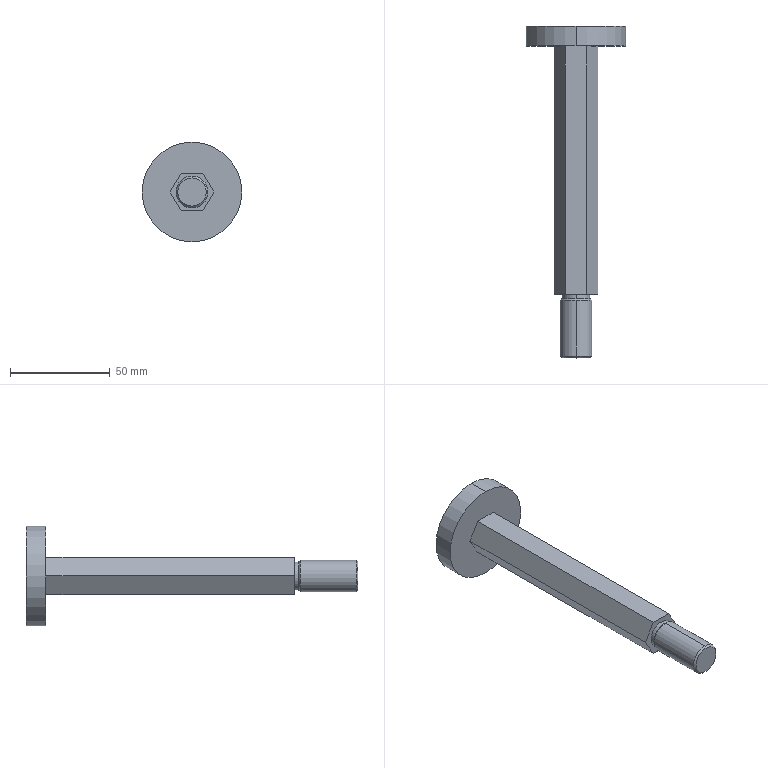Part | SolidWorks | features BaseBody 1 | 1 solid | 21 faces | box 50 x 166.5 x 50 mm | volume 64845 mm3 | plane 11 | cylinder 6 | cone 4 | commonest cylinder face diameters 14 x2 16 x2 50 x2
STEP:
#1=CARTESIAN_POINT('',(225.,248.5,159.621));
#2=VERTEX_POINT('',#1);
#3=CARTESIAN_POINT('',(225.,248.5,109.621));
#4=VERTEX_POINT('',#3);
#5=CARTESIAN_POINT('',(225.,248.5,134.621));
#6=DIRECTION('',(0.,1.,0.));
#7=DIRECTION('',(0.,0.,1.));
#8=AXIS2_PLACEMENT_3D('',#5,#6,#7);
#9=CIRCLE('',#8,25.);
#10=EDGE_CURVE('',#2,#4,#9,.T.);
#11=ORIENTED_EDGE('',*,*,#10,.T.);
#12=CARTESIAN_POINT('',(225.,258.5,109.621));
#13=VERTEX_POINT('',#12);
#14=CARTESIAN_POINT('',(225.,253.5,109.621));
#15=DIRECTION('',(0.,1.,0.));
#16=VECTOR('',#15,1000.);
#17=LINE('',#14,#16);
#18=EDGE_CURVE('',#4,#13,#17,.T.);
#19=ORIENTED_EDGE('',*,*,#18,.T.);
#20=CARTESIAN_POINT('',(225.,258.5,159.621));
#21=VERTEX_POINT('',#20);
#22=CARTESIAN_POINT('',(225.,258.5,134.621));
#23=DIRECTION('',(0.,1.,0.));
#24=DIRECTION('',(0.,0.,1.));
#25=AXIS2_PLACEMENT_3D('',#22,#23,#24);
#26=CIRCLE('',#25,25.);
#27=EDGE_CURVE('',#21,#13,#26,.T.);
#28=ORIENTED_EDGE('',*,*,#27,.F.);
#29=CARTESIAN_POINT('',(225.,253.5,159.621));
#30=DIRECTION('',(0.,1.,0.));
#31=VECTOR('',#30,1000.);
#32=LINE('',#29,#31);
#33=EDGE_CURVE('',#2,#21,#32,.T.);
#34=ORIENTED_EDGE('',*,*,#33,.F.);
#35=EDGE_LOOP('',(#11,#19,#28,#34));
#36=FACE_OUTER_BOUND('',#35,.T.);
#37=CARTESIAN_POINT('',(225.,253.5,134.621));
#38=DIRECTION('',(0.,1.,0.));
#39=DIRECTION('',(0.,0.,1.));
#40=AXIS2_PLACEMENT_3D('',#37,#38,#39);
#41=CYLINDRICAL_SURFACE('',#40,25.);
#42=ADVANCED_FACE('',(#36),#41,.T.);
#43=CARTESIAN_POINT('',(225.,121.75,141.621));
#44=VERTEX_POINT('',#43);
#45=CARTESIAN_POINT('',(225.,121.75,127.621));
#46=VERTEX_POINT('',#45);
#47=CARTESIAN_POINT('',(225.,121.75,134.621));
#48=DIRECTION('',(0.,1.,0.));
#49=DIRECTION('',(0.,0.,1.));
#50=AXIS2_PLACEMENT_3D('',#47,#48,#49);
#51=CIRCLE('',#50,7.);
#52=EDGE_CURVE('',#44,#46,#51,.T.);
#53=ORIENTED_EDGE('',*,*,#52,.T.);
#54=CARTESIAN_POINT('',(225.,124.,127.621));
#55=VERTEX_POINT('',#54);
#56=CARTESIAN_POINT('',(225.,122.875,127.621));
#57=DIRECTION('',(0.,1.,0.));
#58=VECTOR('',#57,1000.);
#59=LINE('',#56,#58);
#60=EDGE_CURVE('',#46,#55,#59,.T.);
#61=ORIENTED_EDGE('',*,*,#60,.T.);
#62=CARTESIAN_POINT('',(225.,124.,141.621));
#63=VERTEX_POINT('',#62);
#64=CARTESIAN_POINT('',(225.,124.,134.621));
#65=DIRECTION('',(0.,1.,0.));
#66=DIRECTION('',(0.,0.,1.));
#67=AXIS2_PLACEMENT_3D('',#64,#65,#66);
#68=CIRCLE('',#67,7.);
#69=EDGE_CURVE('',#63,#55,#68,.T.);
#70=ORIENTED_EDGE('',*,*,#69,.F.);
#71=CARTESIAN_POINT('',(225.,122.875,141.621));
#72=DIRECTION('',(0.,1.,0.));
#73=VECTOR('',#72,1000.);
#74=LINE('',#71,#73);
#75=EDGE_CURVE('',#44,#63,#74,.T.);
#76=ORIENTED_EDGE('',*,*,#75,.F.);
#77=EDGE_LOOP('',(#53,#61,#70,#76));
#78=FACE_OUTER_BOUND('',#77,.T.);
#79=CARTESIAN_POINT('',(225.,122.875,134.621));
#80=DIRECTION('',(0.,1.,0.));
#81=DIRECTION('',(0.,0.,1.));
#82=AXIS2_PLACEMENT_3D('',#79,#80,#81);
#83=CYLINDRICAL_SURFACE('',#82,7.);
#84=ADVANCED_FACE('',(#78),#83,.T.);
#85=CARTESIAN_POINT('',(225.,121.75,141.701));
#86=VERTEX_POINT('',#85);
#87=CARTESIAN_POINT('',(225.,121.75,127.541));
#88=VERTEX_POINT('',#87);
#89=CARTESIAN_POINT('',(225.,121.75,134.621));
#90=DIRECTION('',(0.,1.,0.));
#91=DIRECTION('',(0.,0.,-1.));
#92=AXIS2_PLACEMENT_3D('',#89,#90,#91);
#93=CIRCLE('',#92,7.08);
#94=EDGE_CURVE('',#86,#88,#93,.T.);
#95=ORIENTED_EDGE('',*,*,#94,.F.);
#96=CARTESIAN_POINT('',(225.,120.83,142.621));
#97=VERTEX_POINT('',#96);
#98=CARTESIAN_POINT('',(225.,120.83,142.621));
#99=DIRECTION('',(0.,-0.7071,0.7071));
#100=VECTOR('',#99,1000.);
#101=LINE('',#98,#100);
#102=EDGE_CURVE('',#86,#97,#101,.T.);
#103=ORIENTED_EDGE('',*,*,#102,.T.);
#104=CARTESIAN_POINT('',(225.,120.83,126.621));
#105=VERTEX_POINT('',#104);
#106=CARTESIAN_POINT('',(225.,120.83,134.621));
#107=DIRECTION('',(0.,1.,0.));
#108=DIRECTION('',(-0.5,0.,0.866));
#109=AXIS2_PLACEMENT_3D('',#106,#107,#108);
#110=CIRCLE('',#109,8.);
#111=EDGE_CURVE('',#97,#105,#110,.T.);
#112=ORIENTED_EDGE('',*,*,#111,.T.);
#113=CARTESIAN_POINT('',(225.,120.83,126.621));
#114=DIRECTION('',(0.,-0.7071,-0.7071));
#115=VECTOR('',#114,1000.);
#116=LINE('',#113,#115);
#117=EDGE_CURVE('',#88,#105,#116,.T.);
#118=ORIENTED_EDGE('',*,*,#117,.F.);
#119=EDGE_LOOP('',(#95,#103,#112,#118));
#120=FACE_OUTER_BOUND('',#119,.T.);
#121=CARTESIAN_POINT('',(225.,120.83,134.621));
#122=DIRECTION('',(0.,-1.,0.));
#123=DIRECTION('',(0.,0.,-1.));
#124=AXIS2_PLACEMENT_3D('',#121,#122,#123);
#125=CONICAL_SURFACE('',#124,8.,0.7854);
#126=ADVANCED_FACE('',(#120),#125,.T.);
#127=CARTESIAN_POINT('',(225.,92.92,142.621));
#128=VERTEX_POINT('',#127);
#129=CARTESIAN_POINT('',(225.,92.92,126.621));
#130=VERTEX_POINT('',#129);
#131=CARTESIAN_POINT('',(225.,92.92,134.621));
#132=DIRECTION('',(0.,1.,0.));
#133=DIRECTION('',(0.,0.,1.));
#134=AXIS2_PLACEMENT_3D('',#131,#132,#133);
#135=CIRCLE('',#134,8.);
#136=EDGE_CURVE('',#128,#130,#135,.T.);
#137=ORIENTED_EDGE('',*,*,#136,.T.);
#138=CARTESIAN_POINT('',(225.,106.875,126.621));
#139=DIRECTION('',(0.,1.,0.));
#140=VECTOR('',#139,1000.);
#141=LINE('',#138,#140);
#142=EDGE_CURVE('',#130,#105,#141,.T.);
#143=ORIENTED_EDGE('',*,*,#142,.T.);
#144=ORIENTED_EDGE('',*,*,#111,.F.);
#145=CARTESIAN_POINT('',(225.,106.875,142.621));
#146=DIRECTION('',(0.,1.,0.));
#147=VECTOR('',#146,1000.);
#148=LINE('',#145,#147);
#149=EDGE_CURVE('',#128,#97,#148,.T.);
#150=ORIENTED_EDGE('',*,*,#149,.F.);
#151=EDGE_LOOP('',(#137,#143,#144,#150));
#152=FACE_OUTER_BOUND('',#151,.T.);
#153=CARTESIAN_POINT('',(225.,106.875,134.621));
#154=DIRECTION('',(0.,1.,0.));
#155=DIRECTION('',(0.,0.,1.));
#156=AXIS2_PLACEMENT_3D('',#153,#154,#155);
#157=CYLINDRICAL_SURFACE('',#156,8.);
#158=ADVANCED_FACE('',(#152),#157,.T.);
#159=CARTESIAN_POINT('',(225.,92.,141.701));
#160=VERTEX_POINT('',#159);
#161=CARTESIAN_POINT('',(225.,92.,127.541));
#162=VERTEX_POINT('',#161);
#163=CARTESIAN_POINT('',(225.,92.,134.621));
#164=DIRECTION('',(0.,1.,0.));
#165=DIRECTION('',(0.,0.,1.));
#166=AXIS2_PLACEMENT_3D('',#163,#164,#165);
#167=CIRCLE('',#166,7.08);
#168=EDGE_CURVE('',#160,#162,#167,.T.);
#169=ORIENTED_EDGE('',*,*,#168,.T.);
#170=CARTESIAN_POINT('',(225.,92.92,126.621));
#171=DIRECTION('',(0.,0.7071,-0.7071));
#172=VECTOR('',#171,1000.);
#173=LINE('',#170,#172);
#174=EDGE_CURVE('',#162,#130,#173,.T.);
#175=ORIENTED_EDGE('',*,*,#174,.T.);
#176=ORIENTED_EDGE('',*,*,#136,.F.);
#177=CARTESIAN_POINT('',(225.,92.92,142.621));
#178=DIRECTION('',(0.,0.7071,0.7071));
#179=VECTOR('',#178,1000.);
#180=LINE('',#177,#179);
#181=EDGE_CURVE('',#160,#128,#180,.T.);
#182=ORIENTED_EDGE('',*,*,#181,.F.);
#183=EDGE_LOOP('',(#169,#175,#176,#182));
#184=FACE_OUTER_BOUND('',#183,.T.);
#185=CARTESIAN_POINT('',(225.,92.92,134.621));
#186=DIRECTION('',(0.,1.,0.));
#187=DIRECTION('',(0.,0.,1.));
#188=AXIS2_PLACEMENT_3D('',#185,#186,#187);
#189=CONICAL_SURFACE('',#188,8.,0.7854);
#190=ADVANCED_FACE('',(#184),#189,.T.);
#191=ORIENTED_EDGE('',*,*,#27,.T.);
#192=CARTESIAN_POINT('',(225.,258.5,134.621));
#193=DIRECTION('',(0.,1.,0.));
#194=DIRECTION('',(0.,0.,1.));
#195=AXIS2_PLACEMENT_3D('',#192,#193,#194);
#196=CIRCLE('',#195,25.);
#197=EDGE_CURVE('',#13,#21,#196,.T.);
#198=ORIENTED_EDGE('',*,*,#197,.T.);
#199=EDGE_LOOP('',(#191,#198));
#200=FACE_OUTER_BOUND('',#199,.T.);
#201=CARTESIAN_POINT('',(235.825,258.5,140.871));
#202=DIRECTION('',(0.,1.,0.));
#203=DIRECTION('',(0.,0.,1.));
#204=AXIS2_PLACEMENT_3D('',#201,#202,#203);
#205=PLANE('',#204);
#206=ADVANCED_FACE('',(#200),#205,.T.);
#207=ORIENTED_EDGE('',*,*,#18,.F.);
#208=CARTESIAN_POINT('',(225.,248.5,134.621));
#209=DIRECTION('',(0.,1.,0.));
#210=DIRECTION('',(0.,0.,1.));
#211=AXIS2_PLACEMENT_3D('',#208,#209,#210);
#212=CIRCLE('',#211,25.);
#213=EDGE_CURVE('',#4,#2,#212,.T.);
#214=ORIENTED_EDGE('',*,*,#213,.T.);
#215=ORIENTED_EDGE('',*,*,#33,.T.);
#216=ORIENTED_EDGE('',*,*,#197,.F.);
#217=EDGE_LOOP('',(#207,#214,#215,#216));
#218=FACE_OUTER_BOUND('',#217,.T.);
#219=CARTESIAN_POINT('',(225.,253.5,134.621));
#220=DIRECTION('',(0.,1.,0.));
#221=DIRECTION('',(0.,0.,1.));
#222=AXIS2_PLACEMENT_3D('',#219,#220,#221);
#223=CYLINDRICAL_SURFACE('',#222,25.);
#224=ADVANCED_FACE('',(#218),#223,.T.);
#225=CARTESIAN_POINT('',(214.03,248.5,134.621));
#226=VERTEX_POINT('',#225);
#227=CARTESIAN_POINT('',(219.515,248.5,144.121));
#228=VERTEX_POINT('',#227);
#229=CARTESIAN_POINT('',(214.03,248.5,134.621));
#230=DIRECTION('',(0.5,0.,0.866));
#231=VECTOR('',#230,1000.);
#232=LINE('',#229,#231);
#233=EDGE_CURVE('',#226,#228,#232,.T.);
#234=ORIENTED_EDGE('',*,*,#233,.T.);
#235=CARTESIAN_POINT('',(230.485,248.5,144.121));
#236=VERTEX_POINT('',#235);
#237=CARTESIAN_POINT('',(242.407,248.5,144.121));
#238=DIRECTION('',(1.,0.,0.));
#239=VECTOR('',#238,1000.);
#240=LINE('',#237,#239);
#241=EDGE_CURVE('',#228,#236,#240,.T.);
#242=ORIENTED_EDGE('',*,*,#241,.T.);
#243=CARTESIAN_POINT('',(235.97,248.5,134.621));
#244=VERTEX_POINT('',#243);
#245=CARTESIAN_POINT('',(230.485,248.5,144.121));
#246=DIRECTION('',(0.5,0.,-0.866));
#247=VECTOR('',#246,1000.);
#248=LINE('',#245,#247);
#249=EDGE_CURVE('',#236,#244,#248,.T.);
#250=ORIENTED_EDGE('',*,*,#249,.T.);
#251=CARTESIAN_POINT('',(230.485,248.5,125.121));
#252=VERTEX_POINT('',#251);
#253=CARTESIAN_POINT('',(235.97,248.5,134.621));
#254=DIRECTION('',(-0.5,0.,-0.866));
#255=VECTOR('',#254,1000.);
#256=LINE('',#253,#255);
#257=EDGE_CURVE('',#244,#252,#256,.T.);
#258=ORIENTED_EDGE('',*,*,#257,.T.);
#259=CARTESIAN_POINT('',(219.515,248.5,125.121));
#260=VERTEX_POINT('',#259);
#261=CARTESIAN_POINT('',(242.407,248.5,125.121));
#262=DIRECTION('',(-1.,0.,0.));
#263=VECTOR('',#262,1000.);
#264=LINE('',#261,#263);
#265=EDGE_CURVE('',#252,#260,#264,.T.);
#266=ORIENTED_EDGE('',*,*,#265,.T.);
#267=CARTESIAN_POINT('',(219.515,248.5,125.121));
#268=DIRECTION('',(-0.5,0.,0.866));
#269=VECTOR('',#268,1000.);
#270=LINE('',#267,#269);
#271=EDGE_CURVE('',#260,#226,#270,.T.);
#272=ORIENTED_EDGE('',*,*,#271,.T.);
#273=EDGE_LOOP('',(#234,#242,#250,#258,#266,#272));
#274=FACE_BOUND('',#273,.T.);
#275=ORIENTED_EDGE('',*,*,#10,.F.);
#276=ORIENTED_EDGE('',*,*,#213,.F.);
#277=EDGE_LOOP('',(#275,#276));
#278=FACE_OUTER_BOUND('',#277,.T.);
#279=CARTESIAN_POINT('',(242.407,248.5,144.671));
#280=DIRECTION('',(0.,-1.,0.));
#281=DIRECTION('',(0.,0.,-1.));
#282=AXIS2_PLACEMENT_3D('',#279,#280,#281);
#283=PLANE('',#282);
#284=ADVANCED_FACE('',(#274,#278),#283,.T.);
#285=CARTESIAN_POINT('',(230.485,124.,144.121));
#286=VERTEX_POINT('',#285);
#287=CARTESIAN_POINT('',(219.515,124.,144.121));
#288=VERTEX_POINT('',#287);
#289=CARTESIAN_POINT('',(219.515,124.,144.121));
#290=DIRECTION('',(-1.,0.,0.));
#291=VECTOR('',#290,1000.);
#292=LINE('',#289,#291);
#293=EDGE_CURVE('',#286,#288,#292,.T.);
#294=ORIENTED_EDGE('',*,*,#293,.F.);
#295=CARTESIAN_POINT('',(230.485,124.,144.121));
#296=DIRECTION('',(0.,-1.,0.));
#297=VECTOR('',#296,1000.);
#298=LINE('',#295,#297);
#299=EDGE_CURVE('',#236,#286,#298,.T.);
#300=ORIENTED_EDGE('',*,*,#299,.F.);
#301=ORIENTED_EDGE('',*,*,#241,.F.);
#302=CARTESIAN_POINT('',(219.515,124.,144.121));
#303=DIRECTION('',(0.,1.,0.));
#304=VECTOR('',#303,1000.);
#305=LINE('',#302,#304);
#306=EDGE_CURVE('',#288,#228,#305,.T.);
#307=ORIENTED_EDGE('',*,*,#306,.F.);
#308=EDGE_LOOP('',(#294,#300,#301,#307));
#309=FACE_OUTER_BOUND('',#308,.T.);
#310=CARTESIAN_POINT('',(219.515,124.,144.121));
#311=DIRECTION('',(0.,0.,-1.));
#312=DIRECTION('',(-1.,0.,0.));
#313=AXIS2_PLACEMENT_3D('',#310,#311,#312);
#314=PLANE('',#313);
#315=ADVANCED_FACE('',(#309),#314,.F.);
#316=CARTESIAN_POINT('',(214.03,124.,134.621));
#317=VERTEX_POINT('',#316);
#318=CARTESIAN_POINT('',(214.03,124.,134.621));
#319=DIRECTION('',(-0.5,0.,-0.866));
#320=VECTOR('',#319,1000.);
#321=LINE('',#318,#320);
#322=EDGE_CURVE('',#288,#317,#321,.T.);
#323=ORIENTED_EDGE('',*,*,#322,.F.);
#324=ORIENTED_EDGE('',*,*,#306,.T.);
#325=ORIENTED_EDGE('',*,*,#233,.F.);
#326=CARTESIAN_POINT('',(214.03,124.,134.621));
#327=DIRECTION('',(0.,1.,0.));
#328=VECTOR('',#327,1000.);
#329=LINE('',#326,#328);
#330=EDGE_CURVE('',#317,#226,#329,.T.);
#331=ORIENTED_EDGE('',*,*,#330,.F.);
#332=EDGE_LOOP('',(#323,#324,#325,#331));
#333=FACE_OUTER_BOUND('',#332,.T.);
#334=CARTESIAN_POINT('',(214.03,124.,134.621));
#335=DIRECTION('',(0.866,0.,-0.5));
#336=DIRECTION('',(-0.5,0.,-0.866));
#337=AXIS2_PLACEMENT_3D('',#334,#335,#336);
#338=PLANE('',#337);
#339=ADVANCED_FACE('',(#333),#338,.F.);
#340=CARTESIAN_POINT('',(219.515,124.,125.121));
#341=VERTEX_POINT('',#340);
#342=CARTESIAN_POINT('',(219.515,124.,125.121));
#343=DIRECTION('',(0.5,0.,-0.866));
#344=VECTOR('',#343,1000.);
#345=LINE('',#342,#344);
#346=EDGE_CURVE('',#317,#341,#345,.T.);
#347=ORIENTED_EDGE('',*,*,#346,.F.);
#348=ORIENTED_EDGE('',*,*,#330,.T.);
#349=ORIENTED_EDGE('',*,*,#271,.F.);
#350=CARTESIAN_POINT('',(219.515,124.,125.121));
#351=DIRECTION('',(0.,1.,0.));
#352=VECTOR('',#351,1000.);
#353=LINE('',#350,#352);
#354=EDGE_CURVE('',#341,#260,#353,.T.);
#355=ORIENTED_EDGE('',*,*,#354,.F.);
#356=EDGE_LOOP('',(#347,#348,#349,#355));
#357=FACE_OUTER_BOUND('',#356,.T.);
#358=CARTESIAN_POINT('',(219.515,124.,125.121));
#359=DIRECTION('',(0.866,0.,0.5));
#360=DIRECTION('',(0.5,0.,-0.866));
#361=AXIS2_PLACEMENT_3D('',#358,#359,#360);
#362=PLANE('',#361);
#363=ADVANCED_FACE('',(#357),#362,.F.);
#364=CARTESIAN_POINT('',(230.485,124.,125.121));
#365=VERTEX_POINT('',#364);
#366=CARTESIAN_POINT('',(230.485,124.,125.121));
#367=DIRECTION('',(1.,0.,0.));
#368=VECTOR('',#367,1000.);
#369=LINE('',#366,#368);
#370=EDGE_CURVE('',#341,#365,#369,.T.);
#371=ORIENTED_EDGE('',*,*,#370,.F.);
#372=ORIENTED_EDGE('',*,*,#354,.T.);
#373=ORIENTED_EDGE('',*,*,#265,.F.);
#374=CARTESIAN_POINT('',(230.485,124.,125.121));
#375=DIRECTION('',(0.,1.,0.));
#376=VECTOR('',#375,1000.);
#377=LINE('',#374,#376);
#378=EDGE_CURVE('',#365,#252,#377,.T.);
#379=ORIENTED_EDGE('',*,*,#378,.F.);
#380=EDGE_LOOP('',(#371,#372,#373,#379));
#381=FACE_OUTER_BOUND('',#380,.T.);
#382=CARTESIAN_POINT('',(230.485,124.,125.121));
#383=DIRECTION('',(0.,0.,1.));
#384=DIRECTION('',(1.,0.,0.));
#385=AXIS2_PLACEMENT_3D('',#382,#383,#384);
#386=PLANE('',#385);
#387=ADVANCED_FACE('',(#381),#386,.F.);
#388=CARTESIAN_POINT('',(235.97,124.,134.621));
#389=VERTEX_POINT('',#388);
#390=CARTESIAN_POINT('',(235.97,124.,134.621));
#391=DIRECTION('',(0.5,0.,0.866));
#392=VECTOR('',#391,1000.);
#393=LINE('',#390,#392);
#394=EDGE_CURVE('',#365,#389,#393,.T.);
#395=ORIENTED_EDGE('',*,*,#394,.F.);
#396=ORIENTED_EDGE('',*,*,#378,.T.);
#397=ORIENTED_EDGE('',*,*,#257,.F.);
#398=CARTESIAN_POINT('',(235.97,124.,134.621));
#399=DIRECTION('',(0.,1.,0.));
#400=VECTOR('',#399,1000.);
#401=LINE('',#398,#400);
#402=EDGE_CURVE('',#389,#244,#401,.T.);
#403=ORIENTED_EDGE('',*,*,#402,.F.);
#404=EDGE_LOOP('',(#395,#396,#397,#403));
#405=FACE_OUTER_BOUND('',#404,.T.);
#406=CARTESIAN_POINT('',(235.97,124.,134.621));
#407=DIRECTION('',(-0.866,0.,0.5));
#408=DIRECTION('',(0.5,0.,0.866));
#409=AXIS2_PLACEMENT_3D('',#406,#407,#408);
#410=PLANE('',#409);
#411=ADVANCED_FACE('',(#405),#410,.F.);
#412=CARTESIAN_POINT('',(230.485,124.,144.121));
#413=DIRECTION('',(-0.5,0.,0.866));
#414=VECTOR('',#413,1000.);
#415=LINE('',#412,#414);
#416=EDGE_CURVE('',#389,#286,#415,.T.);
#417=ORIENTED_EDGE('',*,*,#416,.F.);
#418=ORIENTED_EDGE('',*,*,#402,.T.);
#419=ORIENTED_EDGE('',*,*,#249,.F.);
#420=ORIENTED_EDGE('',*,*,#299,.T.);
#421=EDGE_LOOP('',(#417,#418,#419,#420));
#422=FACE_OUTER_BOUND('',#421,.T.);
#423=CARTESIAN_POINT('',(230.485,124.,144.121));
#424=DIRECTION('',(-0.866,0.,-0.5));
#425=DIRECTION('',(-0.5,0.,0.866));
#426=AXIS2_PLACEMENT_3D('',#423,#424,#425);
#427=PLANE('',#426);
#428=ADVANCED_FACE('',(#422),#427,.F.);
#429=ORIENTED_EDGE('',*,*,#416,.T.);
#430=ORIENTED_EDGE('',*,*,#293,.T.);
#431=ORIENTED_EDGE('',*,*,#322,.T.);
#432=ORIENTED_EDGE('',*,*,#346,.T.);
#433=ORIENTED_EDGE('',*,*,#370,.T.);
#434=ORIENTED_EDGE('',*,*,#394,.T.);
#435=EDGE_LOOP('',(#429,#430,#431,#432,#433,#434));
#436=FACE_OUTER_BOUND('',#435,.T.);
#437=ORIENTED_EDGE('',*,*,#69,.T.);
#438=CARTESIAN_POINT('',(225.,124.,134.621));
#439=DIRECTION('',(0.,1.,0.));
#440=DIRECTION('',(0.,0.,1.));
#441=AXIS2_PLACEMENT_3D('',#438,#439,#440);
#442=CIRCLE('',#441,7.);
#443=EDGE_CURVE('',#55,#63,#442,.T.);
#444=ORIENTED_EDGE('',*,*,#443,.T.);
#445=EDGE_LOOP('',(#437,#444));
#446=FACE_BOUND('',#445,.T.);
#447=CARTESIAN_POINT('',(234.613,124.,140.171));
#448=DIRECTION('',(0.,-1.,0.));
#449=DIRECTION('',(0.,0.,-1.));
#450=AXIS2_PLACEMENT_3D('',#447,#448,#449);
#451=PLANE('',#450);
#452=ADVANCED_FACE('',(#436,#446),#451,.T.);
#453=ORIENTED_EDGE('',*,*,#60,.F.);
#454=CARTESIAN_POINT('',(225.,121.75,134.621));
#455=DIRECTION('',(0.,1.,0.));
#456=DIRECTION('',(0.,0.,1.));
#457=AXIS2_PLACEMENT_3D('',#454,#455,#456);
#458=CIRCLE('',#457,7.);
#459=EDGE_CURVE('',#46,#44,#458,.T.);
#460=ORIENTED_EDGE('',*,*,#459,.T.);
#461=ORIENTED_EDGE('',*,*,#75,.T.);
#462=ORIENTED_EDGE('',*,*,#443,.F.);
#463=EDGE_LOOP('',(#453,#460,#461,#462));
#464=FACE_OUTER_BOUND('',#463,.T.);
#465=CARTESIAN_POINT('',(225.,122.875,134.621));
#466=DIRECTION('',(0.,1.,0.));
#467=DIRECTION('',(0.,0.,1.));
#468=AXIS2_PLACEMENT_3D('',#465,#466,#467);
#469=CYLINDRICAL_SURFACE('',#468,7.);
#470=ADVANCED_FACE('',(#464),#469,.T.);
#471=CARTESIAN_POINT('',(225.,121.75,134.621));
#472=DIRECTION('',(0.,1.,0.));
#473=DIRECTION('',(0.,0.,-1.));
#474=AXIS2_PLACEMENT_3D('',#471,#472,#473);
#475=CIRCLE('',#474,7.08);
#476=EDGE_CURVE('',#88,#86,#475,.T.);
#477=ORIENTED_EDGE('',*,*,#476,.T.);
#478=ORIENTED_EDGE('',*,*,#94,.T.);
#479=EDGE_LOOP('',(#477,#478));
#480=FACE_OUTER_BOUND('',#479,.T.);
#481=ORIENTED_EDGE('',*,*,#52,.F.);
#482=ORIENTED_EDGE('',*,*,#459,.F.);
#483=EDGE_LOOP('',(#481,#482));
#484=FACE_BOUND('',#483,.T.);
#485=CARTESIAN_POINT('',(231.097,121.75,138.141));
#486=DIRECTION('',(0.,1.,0.));
#487=DIRECTION('',(0.,0.,1.));
#488=AXIS2_PLACEMENT_3D('',#485,#486,#487);
#489=PLANE('',#488);
#490=ADVANCED_FACE('',(#480,#484),#489,.T.);
#491=ORIENTED_EDGE('',*,*,#102,.F.);
#492=ORIENTED_EDGE('',*,*,#476,.F.);
#493=ORIENTED_EDGE('',*,*,#117,.T.);
#494=CARTESIAN_POINT('',(225.,120.83,134.621));
#495=DIRECTION('',(0.,1.,0.));
#496=DIRECTION('',(-0.5,0.,0.866));
#497=AXIS2_PLACEMENT_3D('',#494,#495,#496);
#498=CIRCLE('',#497,8.);
#499=EDGE_CURVE('',#105,#97,#498,.T.);
#500=ORIENTED_EDGE('',*,*,#499,.T.);
#501=EDGE_LOOP('',(#491,#492,#493,#500));
#502=FACE_OUTER_BOUND('',#501,.T.);
#503=CARTESIAN_POINT('',(225.,120.83,134.621));
#504=DIRECTION('',(0.,-1.,0.));
#505=DIRECTION('',(0.,0.,-1.));
#506=AXIS2_PLACEMENT_3D('',#503,#504,#505);
#507=CONICAL_SURFACE('',#506,8.,0.7854);
#508=ADVANCED_FACE('',(#502),#507,.T.);
#509=ORIENTED_EDGE('',*,*,#142,.F.);
#510=CARTESIAN_POINT('',(225.,92.92,134.621));
#511=DIRECTION('',(0.,1.,0.));
#512=DIRECTION('',(0.,0.,1.));
#513=AXIS2_PLACEMENT_3D('',#510,#511,#512);
#514=CIRCLE('',#513,8.);
#515=EDGE_CURVE('',#130,#128,#514,.T.);
#516=ORIENTED_EDGE('',*,*,#515,.T.);
#517=ORIENTED_EDGE('',*,*,#149,.T.);
#518=ORIENTED_EDGE('',*,*,#499,.F.);
#519=EDGE_LOOP('',(#509,#516,#517,#518));
#520=FACE_OUTER_BOUND('',#519,.T.);
#521=CARTESIAN_POINT('',(225.,106.875,134.621));
#522=DIRECTION('',(0.,1.,0.));
#523=DIRECTION('',(0.,0.,1.));
#524=AXIS2_PLACEMENT_3D('',#521,#522,#523);
#525=CYLINDRICAL_SURFACE('',#524,8.);
#526=ADVANCED_FACE('',(#520),#525,.T.);
#527=ORIENTED_EDGE('',*,*,#174,.F.);
#528=CARTESIAN_POINT('',(225.,92.,134.621));
#529=DIRECTION('',(0.,1.,0.));
#530=DIRECTION('',(0.,0.,1.));
#531=AXIS2_PLACEMENT_3D('',#528,#529,#530);
#532=CIRCLE('',#531,7.08);
#533=EDGE_CURVE('',#162,#160,#532,.T.);
#534=ORIENTED_EDGE('',*,*,#533,.T.);
#535=ORIENTED_EDGE('',*,*,#181,.T.);
#536=ORIENTED_EDGE('',*,*,#515,.F.);
#537=EDGE_LOOP('',(#527,#534,#535,#536));
#538=FACE_OUTER_BOUND('',#537,.T.);
#539=CARTESIAN_POINT('',(225.,92.92,134.621));
#540=DIRECTION('',(0.,1.,0.));
#541=DIRECTION('',(0.,0.,1.));
#542=AXIS2_PLACEMENT_3D('',#539,#540,#541);
#543=CONICAL_SURFACE('',#542,8.,0.7854);
#544=ADVANCED_FACE('',(#538),#543,.T.);
#545=ORIENTED_EDGE('',*,*,#168,.F.);
#546=ORIENTED_EDGE('',*,*,#533,.F.);
#547=EDGE_LOOP('',(#545,#546));
#548=FACE_OUTER_BOUND('',#547,.T.);
#549=CARTESIAN_POINT('',(228.066,92.,136.391));
#550=DIRECTION('',(0.,-1.,0.));
#551=DIRECTION('',(0.,0.,-1.));
#552=AXIS2_PLACEMENT_3D('',#549,#550,#551);
#553=PLANE('',#552);
#554=ADVANCED_FACE('',(#548),#553,.T.);
#555=CLOSED_SHELL('',(#42,#84,#126,#158,#190,#206,#224,#284,#315,#339,#363,#387,#411,#428,#452,#470,#490,#508,#526,#544,#554));
#556=MANIFOLD_SOLID_BREP('',#555);
#557=CARTESIAN_POINT('',(0.,0.,0.));
#558=DIRECTION('',(0.,0.,1.));
#559=DIRECTION('',(1.,0.,0.));
#560=AXIS2_PLACEMENT_3D('',#557,#558,#559);
#561=(LENGTH_UNIT()NAMED_UNIT(*)SI_UNIT(.MILLI.,.METRE.));
#562=UNCERTAINTY_MEASURE_WITH_UNIT(LENGTH_MEASURE(0.00001),#561,'','');
#563=(NAMED_UNIT(*)PLANE_ANGLE_UNIT()SI_UNIT($,.RADIAN.));
#564=(NAMED_UNIT(*)SI_UNIT($,.STERADIAN.)SOLID_ANGLE_UNIT());
#565=(GEOMETRIC_REPRESENTATION_CONTEXT(3)GLOBAL_UNCERTAINTY_ASSIGNED_CONTEXT((#562))GLOBAL_UNIT_ASSIGNED_CONTEXT((#561,#563,#564))REPRESENTATION_CONTEXT('',''));
#566=ADVANCED_BREP_SHAPE_REPRESENTATION('',(#556,#560),#565);